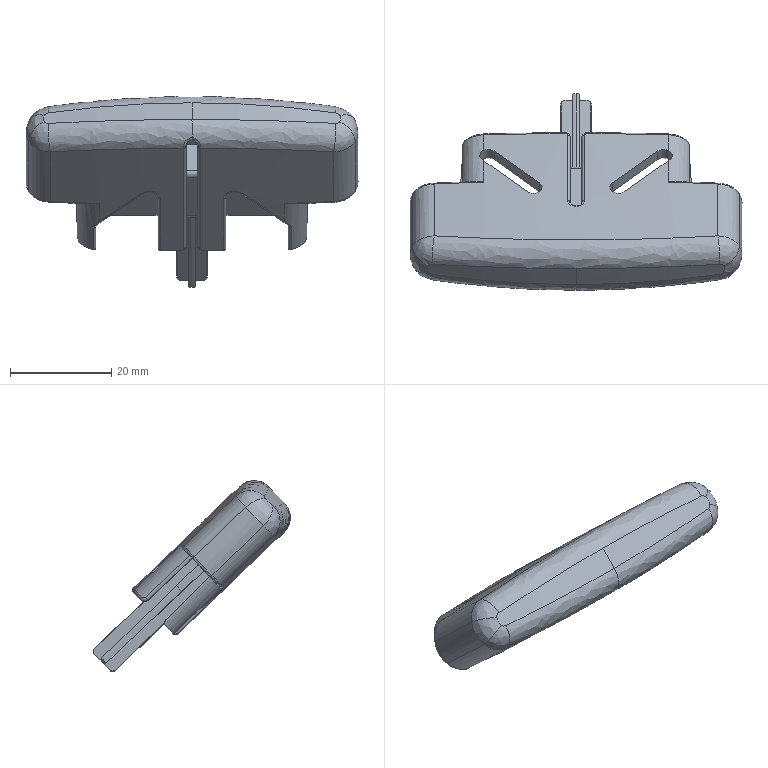Part | SolidWorks | features BaseBody 1 | 1 solid | 238 faces | box 65.6 x 38.87 x 37.679 mm | volume 10434 mm3 | spline 82 | plane 72 | cylinder 65 | cone 19 | commonest cylinder face diameters 1 x13 2 x13 3.3 x12 10 x8 403.238 x8 6 x5